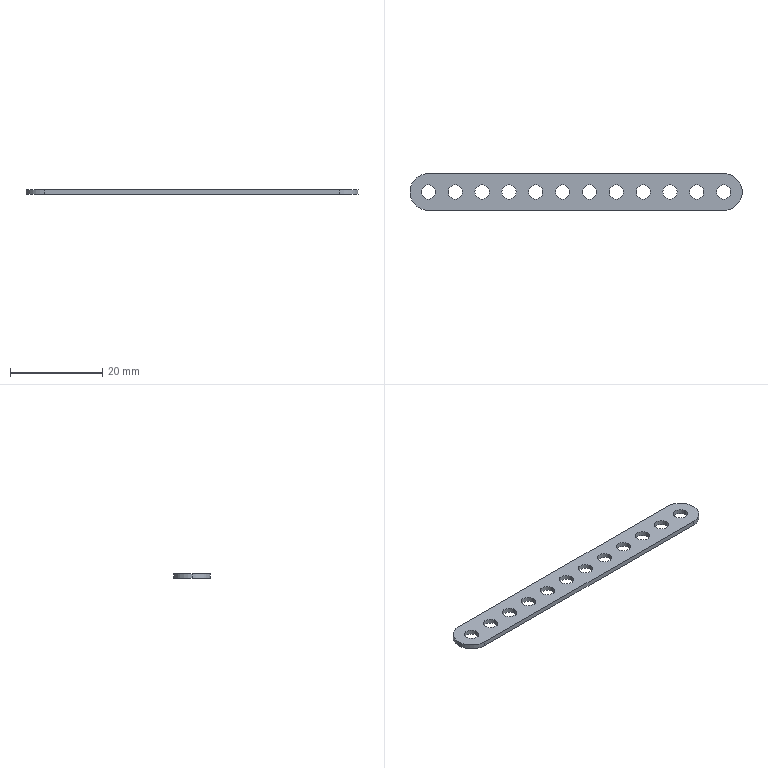Part | SolidWorks | features Extrusion 1 | 1 solid | 31 faces | box 72 x 8 x 1 mm | volume 471.693 mm3 | cylinder 27 | plane 4 | commonest cylinder face diameters 3.1 x24 8 x3
STEP:
#1=CARTESIAN_POINT('',(-4.,0.,1.));
#2=VERTEX_POINT('',#1);
#3=CARTESIAN_POINT('',(0.,-4.,1.));
#4=VERTEX_POINT('',#3);
#5=CARTESIAN_POINT('',(0.,0.,1.));
#6=DIRECTION('',(0.,0.,1.));
#7=DIRECTION('',(1.,0.,0.));
#8=AXIS2_PLACEMENT_3D('',#5,#6,#7);
#9=CIRCLE('',#8,4.);
#10=EDGE_CURVE('',#2,#4,#9,.T.);
#11=ORIENTED_EDGE('',*,*,#10,.F.);
#12=CARTESIAN_POINT('',(-4.,0.,0.));
#13=VERTEX_POINT('',#12);
#14=CARTESIAN_POINT('',(-4.,0.,1.));
#15=DIRECTION('',(0.,0.,-1.));
#16=VECTOR('',#15,1000.);
#17=LINE('',#14,#16);
#18=EDGE_CURVE('',#2,#13,#17,.T.);
#19=ORIENTED_EDGE('',*,*,#18,.T.);
#20=CARTESIAN_POINT('',(0.,-4.,0.));
#21=VERTEX_POINT('',#20);
#22=CARTESIAN_POINT('',(0.,0.,0.));
#23=DIRECTION('',(0.,0.,1.));
#24=DIRECTION('',(1.,0.,0.));
#25=AXIS2_PLACEMENT_3D('',#22,#23,#24);
#26=CIRCLE('',#25,4.);
#27=EDGE_CURVE('',#13,#21,#26,.T.);
#28=ORIENTED_EDGE('',*,*,#27,.T.);
#29=CARTESIAN_POINT('',(0.,-4.,1.));
#30=DIRECTION('',(0.,0.,-1.));
#31=VECTOR('',#30,1000.);
#32=LINE('',#29,#31);
#33=EDGE_CURVE('',#4,#21,#32,.T.);
#34=ORIENTED_EDGE('',*,*,#33,.F.);
#35=EDGE_LOOP('',(#11,#19,#28,#34));
#36=FACE_OUTER_BOUND('',#35,.T.);
#37=CARTESIAN_POINT('',(0.,0.,1.));
#38=DIRECTION('',(0.,0.,-1.));
#39=DIRECTION('',(-1.,0.,0.));
#40=AXIS2_PLACEMENT_3D('',#37,#38,#39);
#41=CYLINDRICAL_SURFACE('',#40,4.);
#42=ADVANCED_FACE('',(#36),#41,.T.);
#43=CARTESIAN_POINT('',(4.268,0.,1.));
#44=VERTEX_POINT('',#43);
#45=CARTESIAN_POINT('',(7.368,0.,1.));
#46=VERTEX_POINT('',#45);
#47=CARTESIAN_POINT('',(5.818,0.,1.));
#48=DIRECTION('',(0.,0.,1.));
#49=DIRECTION('',(1.,0.,0.));
#50=AXIS2_PLACEMENT_3D('',#47,#48,#49);
#51=CIRCLE('',#50,1.55);
#52=EDGE_CURVE('',#44,#46,#51,.T.);
#53=ORIENTED_EDGE('',*,*,#52,.T.);
#54=CARTESIAN_POINT('',(7.368,0.,0.));
#55=VERTEX_POINT('',#54);
#56=CARTESIAN_POINT('',(7.368,0.,1.));
#57=DIRECTION('',(0.,0.,-1.));
#58=VECTOR('',#57,1000.);
#59=LINE('',#56,#58);
#60=EDGE_CURVE('',#46,#55,#59,.T.);
#61=ORIENTED_EDGE('',*,*,#60,.T.);
#62=CARTESIAN_POINT('',(4.268,0.,0.));
#63=VERTEX_POINT('',#62);
#64=CARTESIAN_POINT('',(5.818,0.,0.));
#65=DIRECTION('',(0.,0.,1.));
#66=DIRECTION('',(1.,0.,0.));
#67=AXIS2_PLACEMENT_3D('',#64,#65,#66);
#68=CIRCLE('',#67,1.55);
#69=EDGE_CURVE('',#63,#55,#68,.T.);
#70=ORIENTED_EDGE('',*,*,#69,.F.);
#71=CARTESIAN_POINT('',(4.268,0.,1.));
#72=DIRECTION('',(0.,0.,-1.));
#73=VECTOR('',#72,1000.);
#74=LINE('',#71,#73);
#75=EDGE_CURVE('',#44,#63,#74,.T.);
#76=ORIENTED_EDGE('',*,*,#75,.F.);
#77=EDGE_LOOP('',(#53,#61,#70,#76));
#78=FACE_OUTER_BOUND('',#77,.T.);
#79=CARTESIAN_POINT('',(5.818,0.,1.));
#80=DIRECTION('',(0.,0.,-1.));
#81=DIRECTION('',(-1.,0.,0.));
#82=AXIS2_PLACEMENT_3D('',#79,#80,#81);
#83=CYLINDRICAL_SURFACE('',#82,1.55);
#84=ADVANCED_FACE('',(#78),#83,.F.);
#85=CARTESIAN_POINT('',(10.086,0.,1.));
#86=VERTEX_POINT('',#85);
#87=CARTESIAN_POINT('',(13.186,0.,1.));
#88=VERTEX_POINT('',#87);
#89=CARTESIAN_POINT('',(11.636,0.,1.));
#90=DIRECTION('',(0.,0.,1.));
#91=DIRECTION('',(1.,0.,0.));
#92=AXIS2_PLACEMENT_3D('',#89,#90,#91);
#93=CIRCLE('',#92,1.55);
#94=EDGE_CURVE('',#86,#88,#93,.T.);
#95=ORIENTED_EDGE('',*,*,#94,.T.);
#96=CARTESIAN_POINT('',(13.186,0.,0.));
#97=VERTEX_POINT('',#96);
#98=CARTESIAN_POINT('',(13.186,0.,1.));
#99=DIRECTION('',(0.,0.,-1.));
#100=VECTOR('',#99,1000.);
#101=LINE('',#98,#100);
#102=EDGE_CURVE('',#88,#97,#101,.T.);
#103=ORIENTED_EDGE('',*,*,#102,.T.);
#104=CARTESIAN_POINT('',(10.086,0.,0.));
#105=VERTEX_POINT('',#104);
#106=CARTESIAN_POINT('',(11.636,0.,0.));
#107=DIRECTION('',(0.,0.,1.));
#108=DIRECTION('',(1.,0.,0.));
#109=AXIS2_PLACEMENT_3D('',#106,#107,#108);
#110=CIRCLE('',#109,1.55);
#111=EDGE_CURVE('',#105,#97,#110,.T.);
#112=ORIENTED_EDGE('',*,*,#111,.F.);
#113=CARTESIAN_POINT('',(10.086,0.,1.));
#114=DIRECTION('',(0.,0.,-1.));
#115=VECTOR('',#114,1000.);
#116=LINE('',#113,#115);
#117=EDGE_CURVE('',#86,#105,#116,.T.);
#118=ORIENTED_EDGE('',*,*,#117,.F.);
#119=EDGE_LOOP('',(#95,#103,#112,#118));
#120=FACE_OUTER_BOUND('',#119,.T.);
#121=CARTESIAN_POINT('',(11.636,0.,1.));
#122=DIRECTION('',(0.,0.,-1.));
#123=DIRECTION('',(-1.,0.,0.));
#124=AXIS2_PLACEMENT_3D('',#121,#122,#123);
#125=CYLINDRICAL_SURFACE('',#124,1.55);
#126=ADVANCED_FACE('',(#120),#125,.F.);
#127=CARTESIAN_POINT('',(15.905,0.,1.));
#128=VERTEX_POINT('',#127);
#129=CARTESIAN_POINT('',(19.005,0.,1.));
#130=VERTEX_POINT('',#129);
#131=CARTESIAN_POINT('',(17.455,0.,1.));
#132=DIRECTION('',(0.,0.,1.));
#133=DIRECTION('',(1.,0.,0.));
#134=AXIS2_PLACEMENT_3D('',#131,#132,#133);
#135=CIRCLE('',#134,1.55);
#136=EDGE_CURVE('',#128,#130,#135,.T.);
#137=ORIENTED_EDGE('',*,*,#136,.T.);
#138=CARTESIAN_POINT('',(19.005,0.,0.));
#139=VERTEX_POINT('',#138);
#140=CARTESIAN_POINT('',(19.005,0.,1.));
#141=DIRECTION('',(0.,0.,-1.));
#142=VECTOR('',#141,1000.);
#143=LINE('',#140,#142);
#144=EDGE_CURVE('',#130,#139,#143,.T.);
#145=ORIENTED_EDGE('',*,*,#144,.T.);
#146=CARTESIAN_POINT('',(15.905,0.,0.));
#147=VERTEX_POINT('',#146);
#148=CARTESIAN_POINT('',(17.455,0.,0.));
#149=DIRECTION('',(0.,0.,1.));
#150=DIRECTION('',(1.,0.,0.));
#151=AXIS2_PLACEMENT_3D('',#148,#149,#150);
#152=CIRCLE('',#151,1.55);
#153=EDGE_CURVE('',#147,#139,#152,.T.);
#154=ORIENTED_EDGE('',*,*,#153,.F.);
#155=CARTESIAN_POINT('',(15.905,0.,1.));
#156=DIRECTION('',(0.,0.,-1.));
#157=VECTOR('',#156,1000.);
#158=LINE('',#155,#157);
#159=EDGE_CURVE('',#128,#147,#158,.T.);
#160=ORIENTED_EDGE('',*,*,#159,.F.);
#161=EDGE_LOOP('',(#137,#145,#154,#160));
#162=FACE_OUTER_BOUND('',#161,.T.);
#163=CARTESIAN_POINT('',(17.455,0.,1.));
#164=DIRECTION('',(0.,0.,-1.));
#165=DIRECTION('',(-1.,0.,0.));
#166=AXIS2_PLACEMENT_3D('',#163,#164,#165);
#167=CYLINDRICAL_SURFACE('',#166,1.55);
#168=ADVANCED_FACE('',(#162),#167,.F.);
#169=CARTESIAN_POINT('',(21.723,0.,1.));
#170=VERTEX_POINT('',#169);
#171=CARTESIAN_POINT('',(24.823,0.,1.));
#172=VERTEX_POINT('',#171);
#173=CARTESIAN_POINT('',(23.273,0.,1.));
#174=DIRECTION('',(0.,0.,1.));
#175=DIRECTION('',(1.,0.,0.));
#176=AXIS2_PLACEMENT_3D('',#173,#174,#175);
#177=CIRCLE('',#176,1.55);
#178=EDGE_CURVE('',#170,#172,#177,.T.);
#179=ORIENTED_EDGE('',*,*,#178,.T.);
#180=CARTESIAN_POINT('',(24.823,0.,0.));
#181=VERTEX_POINT('',#180);
#182=CARTESIAN_POINT('',(24.823,0.,1.));
#183=DIRECTION('',(0.,0.,-1.));
#184=VECTOR('',#183,1000.);
#185=LINE('',#182,#184);
#186=EDGE_CURVE('',#172,#181,#185,.T.);
#187=ORIENTED_EDGE('',*,*,#186,.T.);
#188=CARTESIAN_POINT('',(21.723,0.,0.));
#189=VERTEX_POINT('',#188);
#190=CARTESIAN_POINT('',(23.273,0.,0.));
#191=DIRECTION('',(0.,0.,1.));
#192=DIRECTION('',(1.,0.,0.));
#193=AXIS2_PLACEMENT_3D('',#190,#191,#192);
#194=CIRCLE('',#193,1.55);
#195=EDGE_CURVE('',#189,#181,#194,.T.);
#196=ORIENTED_EDGE('',*,*,#195,.F.);
#197=CARTESIAN_POINT('',(21.723,0.,1.));
#198=DIRECTION('',(0.,0.,-1.));
#199=VECTOR('',#198,1000.);
#200=LINE('',#197,#199);
#201=EDGE_CURVE('',#170,#189,#200,.T.);
#202=ORIENTED_EDGE('',*,*,#201,.F.);
#203=EDGE_LOOP('',(#179,#187,#196,#202));
#204=FACE_OUTER_BOUND('',#203,.T.);
#205=CARTESIAN_POINT('',(23.273,0.,1.));
#206=DIRECTION('',(0.,0.,-1.));
#207=DIRECTION('',(-1.,0.,0.));
#208=AXIS2_PLACEMENT_3D('',#205,#206,#207);
#209=CYLINDRICAL_SURFACE('',#208,1.55);
#210=ADVANCED_FACE('',(#204),#209,.F.);
#211=CARTESIAN_POINT('',(27.541,0.,1.));
#212=VERTEX_POINT('',#211);
#213=CARTESIAN_POINT('',(30.641,0.,1.));
#214=VERTEX_POINT('',#213);
#215=CARTESIAN_POINT('',(29.091,0.,1.));
#216=DIRECTION('',(0.,0.,1.));
#217=DIRECTION('',(1.,0.,0.));
#218=AXIS2_PLACEMENT_3D('',#215,#216,#217);
#219=CIRCLE('',#218,1.55);
#220=EDGE_CURVE('',#212,#214,#219,.T.);
#221=ORIENTED_EDGE('',*,*,#220,.T.);
#222=CARTESIAN_POINT('',(30.641,0.,0.));
#223=VERTEX_POINT('',#222);
#224=CARTESIAN_POINT('',(30.641,0.,1.));
#225=DIRECTION('',(0.,0.,-1.));
#226=VECTOR('',#225,1000.);
#227=LINE('',#224,#226);
#228=EDGE_CURVE('',#214,#223,#227,.T.);
#229=ORIENTED_EDGE('',*,*,#228,.T.);
#230=CARTESIAN_POINT('',(27.541,0.,0.));
#231=VERTEX_POINT('',#230);
#232=CARTESIAN_POINT('',(29.091,0.,0.));
#233=DIRECTION('',(0.,0.,1.));
#234=DIRECTION('',(1.,0.,0.));
#235=AXIS2_PLACEMENT_3D('',#232,#233,#234);
#236=CIRCLE('',#235,1.55);
#237=EDGE_CURVE('',#231,#223,#236,.T.);
#238=ORIENTED_EDGE('',*,*,#237,.F.);
#239=CARTESIAN_POINT('',(27.541,0.,1.));
#240=DIRECTION('',(0.,0.,-1.));
#241=VECTOR('',#240,1000.);
#242=LINE('',#239,#241);
#243=EDGE_CURVE('',#212,#231,#242,.T.);
#244=ORIENTED_EDGE('',*,*,#243,.F.);
#245=EDGE_LOOP('',(#221,#229,#238,#244));
#246=FACE_OUTER_BOUND('',#245,.T.);
#247=CARTESIAN_POINT('',(29.091,0.,1.));
#248=DIRECTION('',(0.,0.,-1.));
#249=DIRECTION('',(-1.,0.,0.));
#250=AXIS2_PLACEMENT_3D('',#247,#248,#249);
#251=CYLINDRICAL_SURFACE('',#250,1.55);
#252=ADVANCED_FACE('',(#246),#251,.F.);
#253=CARTESIAN_POINT('',(33.359,0.,1.));
#254=VERTEX_POINT('',#253);
#255=CARTESIAN_POINT('',(36.459,0.,1.));
#256=VERTEX_POINT('',#255);
#257=CARTESIAN_POINT('',(34.909,0.,1.));
#258=DIRECTION('',(0.,0.,1.));
#259=DIRECTION('',(1.,0.,0.));
#260=AXIS2_PLACEMENT_3D('',#257,#258,#259);
#261=CIRCLE('',#260,1.55);
#262=EDGE_CURVE('',#254,#256,#261,.T.);
#263=ORIENTED_EDGE('',*,*,#262,.T.);
#264=CARTESIAN_POINT('',(36.459,0.,0.));
#265=VERTEX_POINT('',#264);
#266=CARTESIAN_POINT('',(36.459,0.,1.));
#267=DIRECTION('',(0.,0.,-1.));
#268=VECTOR('',#267,1000.);
#269=LINE('',#266,#268);
#270=EDGE_CURVE('',#256,#265,#269,.T.);
#271=ORIENTED_EDGE('',*,*,#270,.T.);
#272=CARTESIAN_POINT('',(33.359,0.,0.));
#273=VERTEX_POINT('',#272);
#274=CARTESIAN_POINT('',(34.909,0.,0.));
#275=DIRECTION('',(0.,0.,1.));
#276=DIRECTION('',(1.,0.,0.));
#277=AXIS2_PLACEMENT_3D('',#274,#275,#276);
#278=CIRCLE('',#277,1.55);
#279=EDGE_CURVE('',#273,#265,#278,.T.);
#280=ORIENTED_EDGE('',*,*,#279,.F.);
#281=CARTESIAN_POINT('',(33.359,0.,1.));
#282=DIRECTION('',(0.,0.,-1.));
#283=VECTOR('',#282,1000.);
#284=LINE('',#281,#283);
#285=EDGE_CURVE('',#254,#273,#284,.T.);
#286=ORIENTED_EDGE('',*,*,#285,.F.);
#287=EDGE_LOOP('',(#263,#271,#280,#286));
#288=FACE_OUTER_BOUND('',#287,.T.);
#289=CARTESIAN_POINT('',(34.909,0.,1.));
#290=DIRECTION('',(0.,0.,-1.));
#291=DIRECTION('',(-1.,0.,0.));
#292=AXIS2_PLACEMENT_3D('',#289,#290,#291);
#293=CYLINDRICAL_SURFACE('',#292,1.55);
#294=ADVANCED_FACE('',(#288),#293,.F.);
#295=CARTESIAN_POINT('',(39.177,0.,1.));
#296=VERTEX_POINT('',#295);
#297=CARTESIAN_POINT('',(42.277,0.,1.));
#298=VERTEX_POINT('',#297);
#299=CARTESIAN_POINT('',(40.727,0.,1.));
#300=DIRECTION('',(0.,0.,1.));
#301=DIRECTION('',(1.,0.,0.));
#302=AXIS2_PLACEMENT_3D('',#299,#300,#301);
#303=CIRCLE('',#302,1.55);
#304=EDGE_CURVE('',#296,#298,#303,.T.);
#305=ORIENTED_EDGE('',*,*,#304,.T.);
#306=CARTESIAN_POINT('',(42.277,0.,0.));
#307=VERTEX_POINT('',#306);
#308=CARTESIAN_POINT('',(42.277,0.,1.));
#309=DIRECTION('',(0.,0.,-1.));
#310=VECTOR('',#309,1000.);
#311=LINE('',#308,#310);
#312=EDGE_CURVE('',#298,#307,#311,.T.);
#313=ORIENTED_EDGE('',*,*,#312,.T.);
#314=CARTESIAN_POINT('',(39.177,0.,0.));
#315=VERTEX_POINT('',#314);
#316=CARTESIAN_POINT('',(40.727,0.,0.));
#317=DIRECTION('',(0.,0.,1.));
#318=DIRECTION('',(1.,0.,0.));
#319=AXIS2_PLACEMENT_3D('',#316,#317,#318);
#320=CIRCLE('',#319,1.55);
#321=EDGE_CURVE('',#315,#307,#320,.T.);
#322=ORIENTED_EDGE('',*,*,#321,.F.);
#323=CARTESIAN_POINT('',(39.177,0.,1.));
#324=DIRECTION('',(0.,0.,-1.));
#325=VECTOR('',#324,1000.);
#326=LINE('',#323,#325);
#327=EDGE_CURVE('',#296,#315,#326,.T.);
#328=ORIENTED_EDGE('',*,*,#327,.F.);
#329=EDGE_LOOP('',(#305,#313,#322,#328));
#330=FACE_OUTER_BOUND('',#329,.T.);
#331=CARTESIAN_POINT('',(40.727,0.,1.));
#332=DIRECTION('',(0.,0.,-1.));
#333=DIRECTION('',(-1.,0.,0.));
#334=AXIS2_PLACEMENT_3D('',#331,#332,#333);
#335=CYLINDRICAL_SURFACE('',#334,1.55);
#336=ADVANCED_FACE('',(#330),#335,.F.);
#337=CARTESIAN_POINT('',(44.995,0.,1.));
#338=VERTEX_POINT('',#337);
#339=CARTESIAN_POINT('',(48.095,0.,1.));
#340=VERTEX_POINT('',#339);
#341=CARTESIAN_POINT('',(46.545,0.,1.));
#342=DIRECTION('',(0.,0.,1.));
#343=DIRECTION('',(1.,0.,0.));
#344=AXIS2_PLACEMENT_3D('',#341,#342,#343);
#345=CIRCLE('',#344,1.55);
#346=EDGE_CURVE('',#338,#340,#345,.T.);
#347=ORIENTED_EDGE('',*,*,#346,.T.);
#348=CARTESIAN_POINT('',(48.095,0.,0.));
#349=VERTEX_POINT('',#348);
#350=CARTESIAN_POINT('',(48.095,0.,1.));
#351=DIRECTION('',(0.,0.,-1.));
#352=VECTOR('',#351,1000.);
#353=LINE('',#350,#352);
#354=EDGE_CURVE('',#340,#349,#353,.T.);
#355=ORIENTED_EDGE('',*,*,#354,.T.);
#356=CARTESIAN_POINT('',(44.995,0.,0.));
#357=VERTEX_POINT('',#356);
#358=CARTESIAN_POINT('',(46.545,0.,0.));
#359=DIRECTION('',(0.,0.,1.));
#360=DIRECTION('',(1.,0.,0.));
#361=AXIS2_PLACEMENT_3D('',#358,#359,#360);
#362=CIRCLE('',#361,1.55);
#363=EDGE_CURVE('',#357,#349,#362,.T.);
#364=ORIENTED_EDGE('',*,*,#363,.F.);
#365=CARTESIAN_POINT('',(44.995,0.,1.));
#366=DIRECTION('',(0.,0.,-1.));
#367=VECTOR('',#366,1000.);
#368=LINE('',#365,#367);
#369=EDGE_CURVE('',#338,#357,#368,.T.);
#370=ORIENTED_EDGE('',*,*,#369,.F.);
#371=EDGE_LOOP('',(#347,#355,#364,#370));
#372=FACE_OUTER_BOUND('',#371,.T.);
#373=CARTESIAN_POINT('',(46.545,0.,1.));
#374=DIRECTION('',(0.,0.,-1.));
#375=DIRECTION('',(-1.,0.,0.));
#376=AXIS2_PLACEMENT_3D('',#373,#374,#375);
#377=CYLINDRICAL_SURFACE('',#376,1.55);
#378=ADVANCED_FACE('',(#372),#377,.F.);
#379=CARTESIAN_POINT('',(50.814,0.,1.));
#380=VERTEX_POINT('',#379);
#381=CARTESIAN_POINT('',(53.914,0.,1.));
#382=VERTEX_POINT('',#381);
#383=CARTESIAN_POINT('',(52.364,0.,1.));
#384=DIRECTION('',(0.,0.,1.));
#385=DIRECTION('',(1.,0.,0.));
#386=AXIS2_PLACEMENT_3D('',#383,#384,#385);
#387=CIRCLE('',#386,1.55);
#388=EDGE_CURVE('',#380,#382,#387,.T.);
#389=ORIENTED_EDGE('',*,*,#388,.T.);
#390=CARTESIAN_POINT('',(53.914,0.,0.));
#391=VERTEX_POINT('',#390);
#392=CARTESIAN_POINT('',(53.914,0.,1.));
#393=DIRECTION('',(0.,0.,-1.));
#394=VECTOR('',#393,1000.);
#395=LINE('',#392,#394);
#396=EDGE_CURVE('',#382,#391,#395,.T.);
#397=ORIENTED_EDGE('',*,*,#396,.T.);
#398=CARTESIAN_POINT('',(50.814,0.,0.));
#399=VERTEX_POINT('',#398);
#400=CARTESIAN_POINT('',(52.364,0.,0.));
#401=DIRECTION('',(0.,0.,1.));
#402=DIRECTION('',(1.,0.,0.));
#403=AXIS2_PLACEMENT_3D('',#400,#401,#402);
#404=CIRCLE('',#403,1.55);
#405=EDGE_CURVE('',#399,#391,#404,.T.);
#406=ORIENTED_EDGE('',*,*,#405,.F.);
#407=CARTESIAN_POINT('',(50.814,0.,1.));
#408=DIRECTION('',(0.,0.,-1.));
#409=VECTOR('',#408,1000.);
#410=LINE('',#407,#409);
#411=EDGE_CURVE('',#380,#399,#410,.T.);
#412=ORIENTED_EDGE('',*,*,#411,.F.);
#413=EDGE_LOOP('',(#389,#397,#406,#412));
#414=FACE_OUTER_BOUND('',#413,.T.);
#415=CARTESIAN_POINT('',(52.364,0.,1.));
#416=DIRECTION('',(0.,0.,-1.));
#417=DIRECTION('',(-1.,0.,0.));
#418=AXIS2_PLACEMENT_3D('',#415,#416,#417);
#419=CYLINDRICAL_SURFACE('',#418,1.55);
#420=ADVANCED_FACE('',(#414),#419,.F.);
#421=CARTESIAN_POINT('',(56.632,0.,1.));
#422=VERTEX_POINT('',#421);
#423=CARTESIAN_POINT('',(59.732,0.,1.));
#424=VERTEX_POINT('',#423);
#425=CARTESIAN_POINT('',(58.182,0.,1.));
#426=DIRECTION('',(0.,0.,1.));
#427=DIRECTION('',(1.,0.,0.));
#428=AXIS2_PLACEMENT_3D('',#425,#426,#427);
#429=CIRCLE('',#428,1.55);
#430=EDGE_CURVE('',#422,#424,#429,.T.);
#431=ORIENTED_EDGE('',*,*,#430,.T.);
#432=CARTESIAN_POINT('',(59.732,0.,0.));
#433=VERTEX_POINT('',#432);
#434=CARTESIAN_POINT('',(59.732,0.,1.));
#435=DIRECTION('',(0.,0.,-1.));
#436=VECTOR('',#435,1000.);
#437=LINE('',#434,#436);
#438=EDGE_CURVE('',#424,#433,#437,.T.);
#439=ORIENTED_EDGE('',*,*,#438,.T.);
#440=CARTESIAN_POINT('',(56.632,0.,0.));
#441=VERTEX_POINT('',#440);
#442=CARTESIAN_POINT('',(58.182,0.,0.));
#443=DIRECTION('',(0.,0.,1.));
#444=DIRECTION('',(1.,0.,0.));
#445=AXIS2_PLACEMENT_3D('',#442,#443,#444);
#446=CIRCLE('',#445,1.55);
#447=EDGE_CURVE('',#441,#433,#446,.T.);
#448=ORIENTED_EDGE('',*,*,#447,.F.);
#449=CARTESIAN_POINT('',(56.632,0.,1.));
#450=DIRECTION('',(0.,0.,-1.));
#451=VECTOR('',#450,1000.);
#452=LINE('',#449,#451);
#453=EDGE_CURVE('',#422,#441,#452,.T.);
#454=ORIENTED_EDGE('',*,*,#453,.F.);
#455=EDGE_LOOP('',(#431,#439,#448,#454));
#456=FACE_OUTER_BOUND('',#455,.T.);
#457=CARTESIAN_POINT('',(58.182,0.,1.));
#458=DIRECTION('',(0.,0.,-1.));
#459=DIRECTION('',(-1.,0.,0.));
#460=AXIS2_PLACEMENT_3D('',#457,#458,#459);
#461=CYLINDRICAL_SURFACE('',#460,1.55);
#462=ADVANCED_FACE('',(#456),#461,.F.);
#463=CARTESIAN_POINT('',(62.45,0.,1.));
#464=VERTEX_POINT('',#463);
#465=CARTESIAN_POINT('',(65.55,0.,1.));
#466=VERTEX_POINT('',#465);
#467=CARTESIAN_POINT('',(64.,0.,1.));
#468=DIRECTION('',(0.,0.,1.));
#469=DIRECTION('',(1.,0.,0.));
#470=AXIS2_PLACEMENT_3D('',#467,#468,#469);
#471=CIRCLE('',#470,1.55);
#472=EDGE_CURVE('',#464,#466,#471,.T.);
#473=ORIENTED_EDGE('',*,*,#472,.T.);
#474=CARTESIAN_POINT('',(65.55,0.,0.));
#475=VERTEX_POINT('',#474);
#476=CARTESIAN_POINT('',(65.55,0.,1.));
#477=DIRECTION('',(0.,0.,-1.));
#478=VECTOR('',#477,1000.);
#479=LINE('',#476,#478);
#480=EDGE_CURVE('',#466,#475,#479,.T.);
#481=ORIENTED_EDGE('',*,*,#480,.T.);
#482=CARTESIAN_POINT('',(62.45,0.,0.));
#483=VERTEX_POINT('',#482);
#484=CARTESIAN_POINT('',(64.,0.,0.));
#485=DIRECTION('',(0.,0.,1.));
#486=DIRECTION('',(1.,0.,0.));
#487=AXIS2_PLACEMENT_3D('',#484,#485,#486);
#488=CIRCLE('',#487,1.55);
#489=EDGE_CURVE('',#483,#475,#488,.T.);
#490=ORIENTED_EDGE('',*,*,#489,.F.);
#491=CARTESIAN_POINT('',(62.45,0.,1.));
#492=DIRECTION('',(0.,0.,-1.));
#493=VECTOR('',#492,1000.);
#494=LINE('',#491,#493);
#495=EDGE_CURVE('',#464,#483,#494,.T.);
#496=ORIENTED_EDGE('',*,*,#495,.F.);
#497=EDGE_LOOP('',(#473,#481,#490,#496));
#498=FACE_OUTER_BOUND('',#497,.T.);
#499=CARTESIAN_POINT('',(64.,0.,1.));
#500=DIRECTION('',(0.,0.,-1.));
#501=DIRECTION('',(-1.,0.,0.));
#502=AXIS2_PLACEMENT_3D('',#499,#500,#501);
#503=CYLINDRICAL_SURFACE('',#502,1.55);
#504=ADVANCED_FACE('',(#498),#503,.F.);
#505=CARTESIAN_POINT('',(-1.55,0.,1.));
#506=VERTEX_POINT('',#505);
#507=CARTESIAN_POINT('',(1.55,0.,1.));
#508=VERTEX_POINT('',#507);
#509=CARTESIAN_POINT('',(0.,0.,1.));
#510=DIRECTION('',(0.,0.,1.));
#511=DIRECTION('',(1.,0.,0.));
#512=AXIS2_PLACEMENT_3D('',#509,#510,#511);
#513=CIRCLE('',#512,1.55);
#514=EDGE_CURVE('',#506,#508,#513,.T.);
#515=ORIENTED_EDGE('',*,*,#514,.T.);
#516=CARTESIAN_POINT('',(1.55,0.,0.));
#517=VERTEX_POINT('',#516);
#518=CARTESIAN_POINT('',(1.55,0.,1.));
#519=DIRECTION('',(0.,0.,-1.));
#520=VECTOR('',#519,1000.);
#521=LINE('',#518,#520);
#522=EDGE_CURVE('',#508,#517,#521,.T.);
#523=ORIENTED_EDGE('',*,*,#522,.T.);
#524=CARTESIAN_POINT('',(-1.55,0.,0.));
#525=VERTEX_POINT('',#524);
#526=CARTESIAN_POINT('',(0.,0.,0.));
#527=DIRECTION('',(0.,0.,1.));
#528=DIRECTION('',(1.,0.,0.));
#529=AXIS2_PLACEMENT_3D('',#526,#527,#528);
#530=CIRCLE('',#529,1.55);
#531=EDGE_CURVE('',#525,#517,#530,.T.);
#532=ORIENTED_EDGE('',*,*,#531,.F.);
#533=CARTESIAN_POINT('',(-1.55,0.,1.));
#534=DIRECTION('',(0.,0.,-1.));
#535=VECTOR('',#534,1000.);
#536=LINE('',#533,#535);
#537=EDGE_CURVE('',#506,#525,#536,.T.);
#538=ORIENTED_EDGE('',*,*,#537,.F.);
#539=EDGE_LOOP('',(#515,#523,#532,#538));
#540=FACE_OUTER_BOUND('',#539,.T.);
#541=CARTESIAN_POINT('',(0.,0.,1.));
#542=DIRECTION('',(0.,0.,-1.));
#543=DIRECTION('',(-1.,0.,0.));
#544=AXIS2_PLACEMENT_3D('',#541,#542,#543);
#545=CYLINDRICAL_SURFACE('',#544,1.55);
#546=ADVANCED_FACE('',(#540),#545,.F.);
#547=CARTESIAN_POINT('',(64.,-4.,0.));
#548=VERTEX_POINT('',#547);
#549=CARTESIAN_POINT('',(0.,-4.,0.));
#550=DIRECTION('',(1.,0.,0.));
#551=VECTOR('',#550,1000.);
#552=LINE('',#549,#551);
#553=EDGE_CURVE('',#21,#548,#552,.T.);
#554=ORIENTED_EDGE('',*,*,#553,.T.);
#555=CARTESIAN_POINT('',(64.,-4.,1.));
#556=VERTEX_POINT('',#555);
#557=CARTESIAN_POINT('',(64.,-4.,1.));
#558=DIRECTION('',(0.,0.,-1.));
#559=VECTOR('',#558,1000.);
#560=LINE('',#557,#559);
#561=EDGE_CURVE('',#556,#548,#560,.T.);
#562=ORIENTED_EDGE('',*,*,#561,.F.);
#563=CARTESIAN_POINT('',(0.,-4.,1.));
#564=DIRECTION('',(1.,0.,0.));
#565=VECTOR('',#564,1000.);
#566=LINE('',#563,#565);
#567=EDGE_CURVE('',#4,#556,#566,.T.);
#568=ORIENTED_EDGE('',*,*,#567,.F.);
#569=ORIENTED_EDGE('',*,*,#33,.T.);
#570=EDGE_LOOP('',(#554,#562,#568,#569));
#571=FACE_OUTER_BOUND('',#570,.T.);
#572=CARTESIAN_POINT('',(0.,-4.,1.));
#573=DIRECTION('',(0.,1.,0.));
#574=DIRECTION('',(-1.,0.,0.));
#575=AXIS2_PLACEMENT_3D('',#572,#573,#574);
#576=PLANE('',#575);
#577=ADVANCED_FACE('',(#571),#576,.F.);
#578=CARTESIAN_POINT('',(64.,4.,0.));
#579=VERTEX_POINT('',#578);
#580=CARTESIAN_POINT('',(64.,0.,0.));
#581=DIRECTION('',(0.,0.,1.));
#582=DIRECTION('',(1.,0.,0.));
#583=AXIS2_PLACEMENT_3D('',#580,#581,#582);
#584=CIRCLE('',#583,4.);
#585=EDGE_CURVE('',#548,#579,#584,.T.);
#586=ORIENTED_EDGE('',*,*,#585,.T.);
#587=CARTESIAN_POINT('',(64.,4.,1.));
#588=VERTEX_POINT('',#587);
#589=CARTESIAN_POINT('',(64.,4.,1.));
#590=DIRECTION('',(0.,0.,-1.));
#591=VECTOR('',#590,1000.);
#592=LINE('',#589,#591);
#593=EDGE_CURVE('',#588,#579,#592,.T.);
#594=ORIENTED_EDGE('',*,*,#593,.F.);
#595=CARTESIAN_POINT('',(64.,0.,1.));
#596=DIRECTION('',(0.,0.,1.));
#597=DIRECTION('',(1.,0.,0.));
#598=AXIS2_PLACEMENT_3D('',#595,#596,#597);
#599=CIRCLE('',#598,4.);
#600=EDGE_CURVE('',#556,#588,#599,.T.);
#601=ORIENTED_EDGE('',*,*,#600,.F.);
#602=ORIENTED_EDGE('',*,*,#561,.T.);
#603=EDGE_LOOP('',(#586,#594,#601,#602));
#604=FACE_OUTER_BOUND('',#603,.T.);
#605=CARTESIAN_POINT('',(64.,0.,1.));
#606=DIRECTION('',(0.,0.,-1.));
#607=DIRECTION('',(-1.,0.,0.));
#608=AXIS2_PLACEMENT_3D('',#605,#606,#607);
#609=CYLINDRICAL_SURFACE('',#608,4.);
#610=ADVANCED_FACE('',(#604),#609,.T.);
#611=CARTESIAN_POINT('',(0.,4.,0.));
#612=VERTEX_POINT('',#611);
#613=CARTESIAN_POINT('',(0.,4.,0.));
#614=DIRECTION('',(1.,0.,0.));
#615=VECTOR('',#614,1000.);
#616=LINE('',#613,#615);
#617=EDGE_CURVE('',#612,#579,#616,.T.);
#618=ORIENTED_EDGE('',*,*,#617,.F.);
#619=CARTESIAN_POINT('',(0.,4.,1.));
#620=VERTEX_POINT('',#619);
#621=CARTESIAN_POINT('',(0.,4.,1.));
#622=DIRECTION('',(0.,0.,-1.));
#623=VECTOR('',#622,1000.);
#624=LINE('',#621,#623);
#625=EDGE_CURVE('',#620,#612,#624,.T.);
#626=ORIENTED_EDGE('',*,*,#625,.F.);
#627=CARTESIAN_POINT('',(0.,4.,1.));
#628=DIRECTION('',(1.,0.,0.));
#629=VECTOR('',#628,1000.);
#630=LINE('',#627,#629);
#631=EDGE_CURVE('',#620,#588,#630,.T.);
#632=ORIENTED_EDGE('',*,*,#631,.T.);
#633=ORIENTED_EDGE('',*,*,#593,.T.);
#634=EDGE_LOOP('',(#618,#626,#632,#633));
#635=FACE_OUTER_BOUND('',#634,.T.);
#636=CARTESIAN_POINT('',(0.,4.,1.));
#637=DIRECTION('',(0.,1.,0.));
#638=DIRECTION('',(-1.,0.,0.));
#639=AXIS2_PLACEMENT_3D('',#636,#637,#638);
#640=PLANE('',#639);
#641=ADVANCED_FACE('',(#635),#640,.T.);
#642=ORIENTED_EDGE('',*,*,#522,.F.);
#643=CARTESIAN_POINT('',(0.,0.,1.));
#644=DIRECTION('',(0.,0.,1.));
#645=DIRECTION('',(1.,0.,0.));
#646=AXIS2_PLACEMENT_3D('',#643,#644,#645);
#647=CIRCLE('',#646,1.55);
#648=EDGE_CURVE('',#508,#506,#647,.T.);
#649=ORIENTED_EDGE('',*,*,#648,.T.);
#650=ORIENTED_EDGE('',*,*,#537,.T.);
#651=CARTESIAN_POINT('',(0.,0.,0.));
#652=DIRECTION('',(0.,0.,1.));
#653=DIRECTION('',(1.,0.,0.));
#654=AXIS2_PLACEMENT_3D('',#651,#652,#653);
#655=CIRCLE('',#654,1.55);
#656=EDGE_CURVE('',#517,#525,#655,.T.);
#657=ORIENTED_EDGE('',*,*,#656,.F.);
#658=EDGE_LOOP('',(#642,#649,#650,#657));
#659=FACE_OUTER_BOUND('',#658,.T.);
#660=CARTESIAN_POINT('',(0.,0.,1.));
#661=DIRECTION('',(0.,0.,-1.));
#662=DIRECTION('',(-1.,0.,0.));
#663=AXIS2_PLACEMENT_3D('',#660,#661,#662);
#664=CYLINDRICAL_SURFACE('',#663,1.55);
#665=ADVANCED_FACE('',(#659),#664,.F.);
#666=ORIENTED_EDGE('',*,*,#480,.F.);
#667=CARTESIAN_POINT('',(64.,0.,1.));
#668=DIRECTION('',(0.,0.,1.));
#669=DIRECTION('',(1.,0.,0.));
#670=AXIS2_PLACEMENT_3D('',#667,#668,#669);
#671=CIRCLE('',#670,1.55);
#672=EDGE_CURVE('',#466,#464,#671,.T.);
#673=ORIENTED_EDGE('',*,*,#672,.T.);
#674=ORIENTED_EDGE('',*,*,#495,.T.);
#675=CARTESIAN_POINT('',(64.,0.,0.));
#676=DIRECTION('',(0.,0.,1.));
#677=DIRECTION('',(1.,0.,0.));
#678=AXIS2_PLACEMENT_3D('',#675,#676,#677);
#679=CIRCLE('',#678,1.55);
#680=EDGE_CURVE('',#475,#483,#679,.T.);
#681=ORIENTED_EDGE('',*,*,#680,.F.);
#682=EDGE_LOOP('',(#666,#673,#674,#681));
#683=FACE_OUTER_BOUND('',#682,.T.);
#684=CARTESIAN_POINT('',(64.,0.,1.));
#685=DIRECTION('',(0.,0.,-1.));
#686=DIRECTION('',(-1.,0.,0.));
#687=AXIS2_PLACEMENT_3D('',#684,#685,#686);
#688=CYLINDRICAL_SURFACE('',#687,1.55);
#689=ADVANCED_FACE('',(#683),#688,.F.);
#690=ORIENTED_EDGE('',*,*,#438,.F.);
#691=CARTESIAN_POINT('',(58.182,0.,1.));
#692=DIRECTION('',(0.,0.,1.));
#693=DIRECTION('',(1.,0.,0.));
#694=AXIS2_PLACEMENT_3D('',#691,#692,#693);
#695=CIRCLE('',#694,1.55);
#696=EDGE_CURVE('',#424,#422,#695,.T.);
#697=ORIENTED_EDGE('',*,*,#696,.T.);
#698=ORIENTED_EDGE('',*,*,#453,.T.);
#699=CARTESIAN_POINT('',(58.182,0.,0.));
#700=DIRECTION('',(0.,0.,1.));
#701=DIRECTION('',(1.,0.,0.));
#702=AXIS2_PLACEMENT_3D('',#699,#700,#701);
#703=CIRCLE('',#702,1.55);
#704=EDGE_CURVE('',#433,#441,#703,.T.);
#705=ORIENTED_EDGE('',*,*,#704,.F.);
#706=EDGE_LOOP('',(#690,#697,#698,#705));
#707=FACE_OUTER_BOUND('',#706,.T.);
#708=CARTESIAN_POINT('',(58.182,0.,1.));
#709=DIRECTION('',(0.,0.,-1.));
#710=DIRECTION('',(-1.,0.,0.));
#711=AXIS2_PLACEMENT_3D('',#708,#709,#710);
#712=CYLINDRICAL_SURFACE('',#711,1.55);
#713=ADVANCED_FACE('',(#707),#712,.F.);
#714=ORIENTED_EDGE('',*,*,#396,.F.);
#715=CARTESIAN_POINT('',(52.364,0.,1.));
#716=DIRECTION('',(0.,0.,1.));
#717=DIRECTION('',(1.,0.,0.));
#718=AXIS2_PLACEMENT_3D('',#715,#716,#717);
#719=CIRCLE('',#718,1.55);
#720=EDGE_CURVE('',#382,#380,#719,.T.);
#721=ORIENTED_EDGE('',*,*,#720,.T.);
#722=ORIENTED_EDGE('',*,*,#411,.T.);
#723=CARTESIAN_POINT('',(52.364,0.,0.));
#724=DIRECTION('',(0.,0.,1.));
#725=DIRECTION('',(1.,0.,0.));
#726=AXIS2_PLACEMENT_3D('',#723,#724,#725);
#727=CIRCLE('',#726,1.55);
#728=EDGE_CURVE('',#391,#399,#727,.T.);
#729=ORIENTED_EDGE('',*,*,#728,.F.);
#730=EDGE_LOOP('',(#714,#721,#722,#729));
#731=FACE_OUTER_BOUND('',#730,.T.);
#732=CARTESIAN_POINT('',(52.364,0.,1.));
#733=DIRECTION('',(0.,0.,-1.));
#734=DIRECTION('',(-1.,0.,0.));
#735=AXIS2_PLACEMENT_3D('',#732,#733,#734);
#736=CYLINDRICAL_SURFACE('',#735,1.55);
#737=ADVANCED_FACE('',(#731),#736,.F.);
#738=ORIENTED_EDGE('',*,*,#354,.F.);
#739=CARTESIAN_POINT('',(46.545,0.,1.));
#740=DIRECTION('',(0.,0.,1.));
#741=DIRECTION('',(1.,0.,0.));
#742=AXIS2_PLACEMENT_3D('',#739,#740,#741);
#743=CIRCLE('',#742,1.55);
#744=EDGE_CURVE('',#340,#338,#743,.T.);
#745=ORIENTED_EDGE('',*,*,#744,.T.);
#746=ORIENTED_EDGE('',*,*,#369,.T.);
#747=CARTESIAN_POINT('',(46.545,0.,0.));
#748=DIRECTION('',(0.,0.,1.));
#749=DIRECTION('',(1.,0.,0.));
#750=AXIS2_PLACEMENT_3D('',#747,#748,#749);
#751=CIRCLE('',#750,1.55);
#752=EDGE_CURVE('',#349,#357,#751,.T.);
#753=ORIENTED_EDGE('',*,*,#752,.F.);
#754=EDGE_LOOP('',(#738,#745,#746,#753));
#755=FACE_OUTER_BOUND('',#754,.T.);
#756=CARTESIAN_POINT('',(46.545,0.,1.));
#757=DIRECTION('',(0.,0.,-1.));
#758=DIRECTION('',(-1.,0.,0.));
#759=AXIS2_PLACEMENT_3D('',#756,#757,#758);
#760=CYLINDRICAL_SURFACE('',#759,1.55);
#761=ADVANCED_FACE('',(#755),#760,.F.);
#762=ORIENTED_EDGE('',*,*,#312,.F.);
#763=CARTESIAN_POINT('',(40.727,0.,1.));
#764=DIRECTION('',(0.,0.,1.));
#765=DIRECTION('',(1.,0.,0.));
#766=AXIS2_PLACEMENT_3D('',#763,#764,#765);
#767=CIRCLE('',#766,1.55);
#768=EDGE_CURVE('',#298,#296,#767,.T.);
#769=ORIENTED_EDGE('',*,*,#768,.T.);
#770=ORIENTED_EDGE('',*,*,#327,.T.);
#771=CARTESIAN_POINT('',(40.727,0.,0.));
#772=DIRECTION('',(0.,0.,1.));
#773=DIRECTION('',(1.,0.,0.));
#774=AXIS2_PLACEMENT_3D('',#771,#772,#773);
#775=CIRCLE('',#774,1.55);
#776=EDGE_CURVE('',#307,#315,#775,.T.);
#777=ORIENTED_EDGE('',*,*,#776,.F.);
#778=EDGE_LOOP('',(#762,#769,#770,#777));
#779=FACE_OUTER_BOUND('',#778,.T.);
#780=CARTESIAN_POINT('',(40.727,0.,1.));
#781=DIRECTION('',(0.,0.,-1.));
#782=DIRECTION('',(-1.,0.,0.));
#783=AXIS2_PLACEMENT_3D('',#780,#781,#782);
#784=CYLINDRICAL_SURFACE('',#783,1.55);
#785=ADVANCED_FACE('',(#779),#784,.F.);
#786=ORIENTED_EDGE('',*,*,#270,.F.);
#787=CARTESIAN_POINT('',(34.909,0.,1.));
#788=DIRECTION('',(0.,0.,1.));
#789=DIRECTION('',(1.,0.,0.));
#790=AXIS2_PLACEMENT_3D('',#787,#788,#789);
#791=CIRCLE('',#790,1.55);
#792=EDGE_CURVE('',#256,#254,#791,.T.);
#793=ORIENTED_EDGE('',*,*,#792,.T.);
#794=ORIENTED_EDGE('',*,*,#285,.T.);
#795=CARTESIAN_POINT('',(34.909,0.,0.));
#796=DIRECTION('',(0.,0.,1.));
#797=DIRECTION('',(1.,0.,0.));
#798=AXIS2_PLACEMENT_3D('',#795,#796,#797);
#799=CIRCLE('',#798,1.55);
#800=EDGE_CURVE('',#265,#273,#799,.T.);
#801=ORIENTED_EDGE('',*,*,#800,.F.);
#802=EDGE_LOOP('',(#786,#793,#794,#801));
#803=FACE_OUTER_BOUND('',#802,.T.);
#804=CARTESIAN_POINT('',(34.909,0.,1.));
#805=DIRECTION('',(0.,0.,-1.));
#806=DIRECTION('',(-1.,0.,0.));
#807=AXIS2_PLACEMENT_3D('',#804,#805,#806);
#808=CYLINDRICAL_SURFACE('',#807,1.55);
#809=ADVANCED_FACE('',(#803),#808,.F.);
#810=ORIENTED_EDGE('',*,*,#228,.F.);
#811=CARTESIAN_POINT('',(29.091,0.,1.));
#812=DIRECTION('',(0.,0.,1.));
#813=DIRECTION('',(1.,0.,0.));
#814=AXIS2_PLACEMENT_3D('',#811,#812,#813);
#815=CIRCLE('',#814,1.55);
#816=EDGE_CURVE('',#214,#212,#815,.T.);
#817=ORIENTED_EDGE('',*,*,#816,.T.);
#818=ORIENTED_EDGE('',*,*,#243,.T.);
#819=CARTESIAN_POINT('',(29.091,0.,0.));
#820=DIRECTION('',(0.,0.,1.));
#821=DIRECTION('',(1.,0.,0.));
#822=AXIS2_PLACEMENT_3D('',#819,#820,#821);
#823=CIRCLE('',#822,1.55);
#824=EDGE_CURVE('',#223,#231,#823,.T.);
#825=ORIENTED_EDGE('',*,*,#824,.F.);
#826=EDGE_LOOP('',(#810,#817,#818,#825));
#827=FACE_OUTER_BOUND('',#826,.T.);
#828=CARTESIAN_POINT('',(29.091,0.,1.));
#829=DIRECTION('',(0.,0.,-1.));
#830=DIRECTION('',(-1.,0.,0.));
#831=AXIS2_PLACEMENT_3D('',#828,#829,#830);
#832=CYLINDRICAL_SURFACE('',#831,1.55);
#833=ADVANCED_FACE('',(#827),#832,.F.);
#834=ORIENTED_EDGE('',*,*,#186,.F.);
#835=CARTESIAN_POINT('',(23.273,0.,1.));
#836=DIRECTION('',(0.,0.,1.));
#837=DIRECTION('',(1.,0.,0.));
#838=AXIS2_PLACEMENT_3D('',#835,#836,#837);
#839=CIRCLE('',#838,1.55);
#840=EDGE_CURVE('',#172,#170,#839,.T.);
#841=ORIENTED_EDGE('',*,*,#840,.T.);
#842=ORIENTED_EDGE('',*,*,#201,.T.);
#843=CARTESIAN_POINT('',(23.273,0.,0.));
#844=DIRECTION('',(0.,0.,1.));
#845=DIRECTION('',(1.,0.,0.));
#846=AXIS2_PLACEMENT_3D('',#843,#844,#845);
#847=CIRCLE('',#846,1.55);
#848=EDGE_CURVE('',#181,#189,#847,.T.);
#849=ORIENTED_EDGE('',*,*,#848,.F.);
#850=EDGE_LOOP('',(#834,#841,#842,#849));
#851=FACE_OUTER_BOUND('',#850,.T.);
#852=CARTESIAN_POINT('',(23.273,0.,1.));
#853=DIRECTION('',(0.,0.,-1.));
#854=DIRECTION('',(-1.,0.,0.));
#855=AXIS2_PLACEMENT_3D('',#852,#853,#854);
#856=CYLINDRICAL_SURFACE('',#855,1.55);
#857=ADVANCED_FACE('',(#851),#856,.F.);
#858=ORIENTED_EDGE('',*,*,#144,.F.);
#859=CARTESIAN_POINT('',(17.455,0.,1.));
#860=DIRECTION('',(0.,0.,1.));
#861=DIRECTION('',(1.,0.,0.));
#862=AXIS2_PLACEMENT_3D('',#859,#860,#861);
#863=CIRCLE('',#862,1.55);
#864=EDGE_CURVE('',#130,#128,#863,.T.);
#865=ORIENTED_EDGE('',*,*,#864,.T.);
#866=ORIENTED_EDGE('',*,*,#159,.T.);
#867=CARTESIAN_POINT('',(17.455,0.,0.));
#868=DIRECTION('',(0.,0.,1.));
#869=DIRECTION('',(1.,0.,0.));
#870=AXIS2_PLACEMENT_3D('',#867,#868,#869);
#871=CIRCLE('',#870,1.55);
#872=EDGE_CURVE('',#139,#147,#871,.T.);
#873=ORIENTED_EDGE('',*,*,#872,.F.);
#874=EDGE_LOOP('',(#858,#865,#866,#873));
#875=FACE_OUTER_BOUND('',#874,.T.);
#876=CARTESIAN_POINT('',(17.455,0.,1.));
#877=DIRECTION('',(0.,0.,-1.));
#878=DIRECTION('',(-1.,0.,0.));
#879=AXIS2_PLACEMENT_3D('',#876,#877,#878);
#880=CYLINDRICAL_SURFACE('',#879,1.55);
#881=ADVANCED_FACE('',(#875),#880,.F.);
#882=ORIENTED_EDGE('',*,*,#102,.F.);
#883=CARTESIAN_POINT('',(11.636,0.,1.));
#884=DIRECTION('',(0.,0.,1.));
#885=DIRECTION('',(1.,0.,0.));
#886=AXIS2_PLACEMENT_3D('',#883,#884,#885);
#887=CIRCLE('',#886,1.55);
#888=EDGE_CURVE('',#88,#86,#887,.T.);
#889=ORIENTED_EDGE('',*,*,#888,.T.);
#890=ORIENTED_EDGE('',*,*,#117,.T.);
#891=CARTESIAN_POINT('',(11.636,0.,0.));
#892=DIRECTION('',(0.,0.,1.));
#893=DIRECTION('',(1.,0.,0.));
#894=AXIS2_PLACEMENT_3D('',#891,#892,#893);
#895=CIRCLE('',#894,1.55);
#896=EDGE_CURVE('',#97,#105,#895,.T.);
#897=ORIENTED_EDGE('',*,*,#896,.F.);
#898=EDGE_LOOP('',(#882,#889,#890,#897));
#899=FACE_OUTER_BOUND('',#898,.T.);
#900=CARTESIAN_POINT('',(11.636,0.,1.));
#901=DIRECTION('',(0.,0.,-1.));
#902=DIRECTION('',(-1.,0.,0.));
#903=AXIS2_PLACEMENT_3D('',#900,#901,#902);
#904=CYLINDRICAL_SURFACE('',#903,1.55);
#905=ADVANCED_FACE('',(#899),#904,.F.);
#906=ORIENTED_EDGE('',*,*,#60,.F.);
#907=CARTESIAN_POINT('',(5.818,0.,1.));
#908=DIRECTION('',(0.,0.,1.));
#909=DIRECTION('',(1.,0.,0.));
#910=AXIS2_PLACEMENT_3D('',#907,#908,#909);
#911=CIRCLE('',#910,1.55);
#912=EDGE_CURVE('',#46,#44,#911,.T.);
#913=ORIENTED_EDGE('',*,*,#912,.T.);
#914=ORIENTED_EDGE('',*,*,#75,.T.);
#915=CARTESIAN_POINT('',(5.818,0.,0.));
#916=DIRECTION('',(0.,0.,1.));
#917=DIRECTION('',(1.,0.,0.));
#918=AXIS2_PLACEMENT_3D('',#915,#916,#917);
#919=CIRCLE('',#918,1.55);
#920=EDGE_CURVE('',#55,#63,#919,.T.);
#921=ORIENTED_EDGE('',*,*,#920,.F.);
#922=EDGE_LOOP('',(#906,#913,#914,#921));
#923=FACE_OUTER_BOUND('',#922,.T.);
#924=CARTESIAN_POINT('',(5.818,0.,1.));
#925=DIRECTION('',(0.,0.,-1.));
#926=DIRECTION('',(-1.,0.,0.));
#927=AXIS2_PLACEMENT_3D('',#924,#925,#926);
#928=CYLINDRICAL_SURFACE('',#927,1.55);
#929=ADVANCED_FACE('',(#923),#928,.F.);
#930=ORIENTED_EDGE('',*,*,#18,.F.);
#931=CARTESIAN_POINT('',(0.,0.,1.));
#932=DIRECTION('',(0.,0.,1.));
#933=DIRECTION('',(1.,0.,0.));
#934=AXIS2_PLACEMENT_3D('',#931,#932,#933);
#935=CIRCLE('',#934,4.);
#936=EDGE_CURVE('',#620,#2,#935,.T.);
#937=ORIENTED_EDGE('',*,*,#936,.F.);
#938=ORIENTED_EDGE('',*,*,#625,.T.);
#939=CARTESIAN_POINT('',(0.,0.,0.));
#940=DIRECTION('',(0.,0.,1.));
#941=DIRECTION('',(1.,0.,0.));
#942=AXIS2_PLACEMENT_3D('',#939,#940,#941);
#943=CIRCLE('',#942,4.);
#944=EDGE_CURVE('',#612,#13,#943,.T.);
#945=ORIENTED_EDGE('',*,*,#944,.T.);
#946=EDGE_LOOP('',(#930,#937,#938,#945));
#947=FACE_OUTER_BOUND('',#946,.T.);
#948=CARTESIAN_POINT('',(0.,0.,1.));
#949=DIRECTION('',(0.,0.,-1.));
#950=DIRECTION('',(-1.,0.,0.));
#951=AXIS2_PLACEMENT_3D('',#948,#949,#950);
#952=CYLINDRICAL_SURFACE('',#951,4.);
#953=ADVANCED_FACE('',(#947),#952,.T.);
#954=ORIENTED_EDGE('',*,*,#52,.F.);
#955=ORIENTED_EDGE('',*,*,#912,.F.);
#956=EDGE_LOOP('',(#954,#955));
#957=FACE_BOUND('',#956,.T.);
#958=ORIENTED_EDGE('',*,*,#94,.F.);
#959=ORIENTED_EDGE('',*,*,#888,.F.);
#960=EDGE_LOOP('',(#958,#959));
#961=FACE_BOUND('',#960,.T.);
#962=ORIENTED_EDGE('',*,*,#136,.F.);
#963=ORIENTED_EDGE('',*,*,#864,.F.);
#964=EDGE_LOOP('',(#962,#963));
#965=FACE_BOUND('',#964,.T.);
#966=ORIENTED_EDGE('',*,*,#178,.F.);
#967=ORIENTED_EDGE('',*,*,#840,.F.);
#968=EDGE_LOOP('',(#966,#967));
#969=FACE_BOUND('',#968,.T.);
#970=ORIENTED_EDGE('',*,*,#220,.F.);
#971=ORIENTED_EDGE('',*,*,#816,.F.);
#972=EDGE_LOOP('',(#970,#971));
#973=FACE_BOUND('',#972,.T.);
#974=ORIENTED_EDGE('',*,*,#262,.F.);
#975=ORIENTED_EDGE('',*,*,#792,.F.);
#976=EDGE_LOOP('',(#974,#975));
#977=FACE_BOUND('',#976,.T.);
#978=ORIENTED_EDGE('',*,*,#304,.F.);
#979=ORIENTED_EDGE('',*,*,#768,.F.);
#980=EDGE_LOOP('',(#978,#979));
#981=FACE_BOUND('',#980,.T.);
#982=ORIENTED_EDGE('',*,*,#346,.F.);
#983=ORIENTED_EDGE('',*,*,#744,.F.);
#984=EDGE_LOOP('',(#982,#983));
#985=FACE_BOUND('',#984,.T.);
#986=ORIENTED_EDGE('',*,*,#388,.F.);
#987=ORIENTED_EDGE('',*,*,#720,.F.);
#988=EDGE_LOOP('',(#986,#987));
#989=FACE_BOUND('',#988,.T.);
#990=ORIENTED_EDGE('',*,*,#430,.F.);
#991=ORIENTED_EDGE('',*,*,#696,.F.);
#992=EDGE_LOOP('',(#990,#991));
#993=FACE_BOUND('',#992,.T.);
#994=ORIENTED_EDGE('',*,*,#472,.F.);
#995=ORIENTED_EDGE('',*,*,#672,.F.);
#996=EDGE_LOOP('',(#994,#995));
#997=FACE_BOUND('',#996,.T.);
#998=ORIENTED_EDGE('',*,*,#514,.F.);
#999=ORIENTED_EDGE('',*,*,#648,.F.);
#1000=EDGE_LOOP('',(#998,#999));
#1001=FACE_BOUND('',#1000,.T.);
#1002=ORIENTED_EDGE('',*,*,#567,.T.);
#1003=ORIENTED_EDGE('',*,*,#600,.T.);
#1004=ORIENTED_EDGE('',*,*,#631,.F.);
#1005=ORIENTED_EDGE('',*,*,#936,.T.);
#1006=ORIENTED_EDGE('',*,*,#10,.T.);
#1007=EDGE_LOOP('',(#1002,#1003,#1004,#1005,#1006));
#1008=FACE_OUTER_BOUND('',#1007,.T.);
#1009=CARTESIAN_POINT('',(0.,0.,1.));
#1010=DIRECTION('',(0.,0.,1.));
#1011=DIRECTION('',(1.,0.,0.));
#1012=AXIS2_PLACEMENT_3D('',#1009,#1010,#1011);
#1013=PLANE('',#1012);
#1014=ADVANCED_FACE('',(#957,#961,#965,#969,#973,#977,#981,#985,#989,#993,#997,#1001,#1008),#1013,.T.);
#1015=ORIENTED_EDGE('',*,*,#69,.T.);
#1016=ORIENTED_EDGE('',*,*,#920,.T.);
#1017=EDGE_LOOP('',(#1015,#1016));
#1018=FACE_BOUND('',#1017,.T.);
#1019=ORIENTED_EDGE('',*,*,#111,.T.);
#1020=ORIENTED_EDGE('',*,*,#896,.T.);
#1021=EDGE_LOOP('',(#1019,#1020));
#1022=FACE_BOUND('',#1021,.T.);
#1023=ORIENTED_EDGE('',*,*,#153,.T.);
#1024=ORIENTED_EDGE('',*,*,#872,.T.);
#1025=EDGE_LOOP('',(#1023,#1024));
#1026=FACE_BOUND('',#1025,.T.);
#1027=ORIENTED_EDGE('',*,*,#195,.T.);
#1028=ORIENTED_EDGE('',*,*,#848,.T.);
#1029=EDGE_LOOP('',(#1027,#1028));
#1030=FACE_BOUND('',#1029,.T.);
#1031=ORIENTED_EDGE('',*,*,#237,.T.);
#1032=ORIENTED_EDGE('',*,*,#824,.T.);
#1033=EDGE_LOOP('',(#1031,#1032));
#1034=FACE_BOUND('',#1033,.T.);
#1035=ORIENTED_EDGE('',*,*,#279,.T.);
#1036=ORIENTED_EDGE('',*,*,#800,.T.);
#1037=EDGE_LOOP('',(#1035,#1036));
#1038=FACE_BOUND('',#1037,.T.);
#1039=ORIENTED_EDGE('',*,*,#321,.T.);
#1040=ORIENTED_EDGE('',*,*,#776,.T.);
#1041=EDGE_LOOP('',(#1039,#1040));
#1042=FACE_BOUND('',#1041,.T.);
#1043=ORIENTED_EDGE('',*,*,#363,.T.);
#1044=ORIENTED_EDGE('',*,*,#752,.T.);
#1045=EDGE_LOOP('',(#1043,#1044));
#1046=FACE_BOUND('',#1045,.T.);
#1047=ORIENTED_EDGE('',*,*,#405,.T.);
#1048=ORIENTED_EDGE('',*,*,#728,.T.);
#1049=EDGE_LOOP('',(#1047,#1048));
#1050=FACE_BOUND('',#1049,.T.);
#1051=ORIENTED_EDGE('',*,*,#447,.T.);
#1052=ORIENTED_EDGE('',*,*,#704,.T.);
#1053=EDGE_LOOP('',(#1051,#1052));
#1054=FACE_BOUND('',#1053,.T.);
#1055=ORIENTED_EDGE('',*,*,#489,.T.);
#1056=ORIENTED_EDGE('',*,*,#680,.T.);
#1057=EDGE_LOOP('',(#1055,#1056));
#1058=FACE_BOUND('',#1057,.T.);
#1059=ORIENTED_EDGE('',*,*,#531,.T.);
#1060=ORIENTED_EDGE('',*,*,#656,.T.);
#1061=EDGE_LOOP('',(#1059,#1060));
#1062=FACE_BOUND('',#1061,.T.);
#1063=ORIENTED_EDGE('',*,*,#553,.F.);
#1064=ORIENTED_EDGE('',*,*,#27,.F.);
#1065=ORIENTED_EDGE('',*,*,#944,.F.);
#1066=ORIENTED_EDGE('',*,*,#617,.T.);
#1067=ORIENTED_EDGE('',*,*,#585,.F.);
#1068=EDGE_LOOP('',(#1063,#1064,#1065,#1066,#1067));
#1069=FACE_OUTER_BOUND('',#1068,.T.);
#1070=CARTESIAN_POINT('',(0.,0.,0.));
#1071=DIRECTION('',(0.,0.,1.));
#1072=DIRECTION('',(1.,0.,0.));
#1073=AXIS2_PLACEMENT_3D('',#1070,#1071,#1072);
#1074=PLANE('',#1073);
#1075=ADVANCED_FACE('',(#1018,#1022,#1026,#1030,#1034,#1038,#1042,#1046,#1050,#1054,#1058,#1062,#1069),#1074,.F.);
#1076=CLOSED_SHELL('',(#42,#84,#126,#168,#210,#252,#294,#336,#378,#420,#462,#504,#546,#577,#610,#641,#665,#689,#713,#737,#761,#785,#809,#833,#857,#881,#905,#929,#953,#1014,#1075));
#1077=MANIFOLD_SOLID_BREP('',#1076);
#1078=CARTESIAN_POINT('',(0.,0.,0.));
#1079=DIRECTION('',(0.,0.,1.));
#1080=DIRECTION('',(1.,0.,0.));
#1081=AXIS2_PLACEMENT_3D('',#1078,#1079,#1080);
#1082=(LENGTH_UNIT()NAMED_UNIT(*)SI_UNIT(.MILLI.,.METRE.));
#1083=UNCERTAINTY_MEASURE_WITH_UNIT(LENGTH_MEASURE(0.00001),#1082,'','');
#1084=(NAMED_UNIT(*)PLANE_ANGLE_UNIT()SI_UNIT($,.RADIAN.));
#1085=(NAMED_UNIT(*)SI_UNIT($,.STERADIAN.)SOLID_ANGLE_UNIT());
#1086=(GEOMETRIC_REPRESENTATION_CONTEXT(3)GLOBAL_UNCERTAINTY_ASSIGNED_CONTEXT((#1083))GLOBAL_UNIT_ASSIGNED_CONTEXT((#1082,#1084,#1085))REPRESENTATION_CONTEXT('',''));
#1087=ADVANCED_BREP_SHAPE_REPRESENTATION('',(#1077,#1081),#1086);